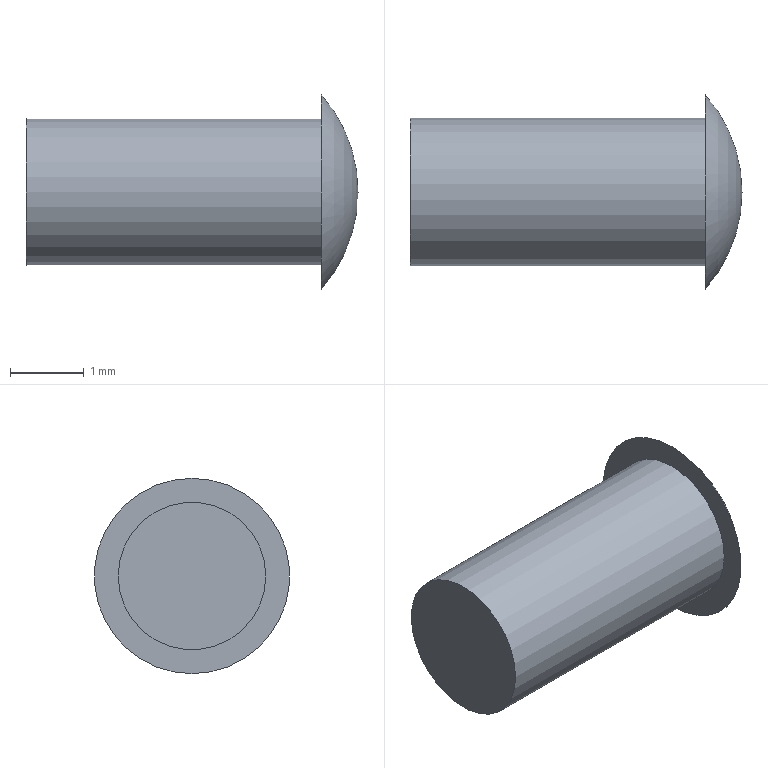Part | STEP file | 1-63部分2毫米Bolt | 1 solid | 4 faces | box 4.5 x 2.646 x 2.646 mm | volume 14.006 mm3 | plane 2 | cylinder 1 | sphere 1 | commonest cylinder face diameters 2 x1
STEP:
#1=CARTESIAN_POINT('',(0.,0.,0.));
#2=DIRECTION('',(0.,0.,1.));
#3=DIRECTION('',(1.,0.,0.));
#4=AXIS2_PLACEMENT_3D('',#1,#2,#3);
#5=CARTESIAN_POINT('',(-2.,1.,0.));
#6=VERTEX_POINT('',#5);
#7=CARTESIAN_POINT('',(-2.,0.,0.));
#8=DIRECTION('',(1.,0.,0.));
#9=DIRECTION('',(0.,1.,0.));
#10=AXIS2_PLACEMENT_3D('',#7,#8,#9);
#11=CIRCLE('',#10,1.);
#12=CARTESIAN_POINT('',(-2.,-0.2679,0.));
#13=DIRECTION('',(1.,0.,0.));
#14=DIRECTION('',(0.,1.,0.));
#15=AXIS2_PLACEMENT_3D('',#12,#13,#14);
#16=PLANE('',#15);
#17=CARTESIAN_POINT('',(0.2679,0.));
#18=DIRECTION('',(1.,0.));
#19=AXIS2_PLACEMENT_2D('',#17,#18);
#20=CIRCLE('',#19,1.);
#21=(GEOMETRIC_REPRESENTATION_CONTEXT(2)PARAMETRIC_REPRESENTATION_CONTEXT()REPRESENTATION_CONTEXT('',''));
#22=DEFINITIONAL_REPRESENTATION('',(#20),#21);
#23=PCURVE('',#16,#22);
#24=CARTESIAN_POINT('',(2.,0.,0.));
#25=DIRECTION('',(-1.,0.,0.));
#26=DIRECTION('',(0.,1.,0.));
#27=AXIS2_PLACEMENT_3D('',#24,#25,#26);
#28=CYLINDRICAL_SURFACE('',#27,1.);
#29=CARTESIAN_POINT('',(6.283,4.));
#30=DIRECTION('',(-1.,0.));
#31=VECTOR('',#30,1.);
#32=LINE('',#29,#31);
#33=(GEOMETRIC_REPRESENTATION_CONTEXT(2)PARAMETRIC_REPRESENTATION_CONTEXT()REPRESENTATION_CONTEXT('',''));
#34=DEFINITIONAL_REPRESENTATION('',(#32),#33);
#35=PCURVE('',#28,#34);
#36=SURFACE_CURVE('',#11,(#23,#35),.PCURVE_S1.);
#37=EDGE_CURVE('',#6,#6,#36,.T.);
#38=ORIENTED_EDGE('',*,*,#37,.T.);
#39=EDGE_LOOP('',(#38));
#40=FACE_BOUND('',#39,.F.);
#41=ADVANCED_FACE('',(#40),#16,.F.);
#42=CARTESIAN_POINT('',(2.,1.,0.));
#43=VERTEX_POINT('',#42);
#44=CARTESIAN_POINT('',(2.,1.,0.));
#45=DIRECTION('',(-1.,0.,0.));
#46=VECTOR('',#45,1.);
#47=LINE('',#44,#46);
#48=CARTESIAN_POINT('',(6.283,0.));
#49=DIRECTION('',(0.,1.));
#50=VECTOR('',#49,1.);
#51=LINE('',#48,#50);
#52=(GEOMETRIC_REPRESENTATION_CONTEXT(2)PARAMETRIC_REPRESENTATION_CONTEXT()REPRESENTATION_CONTEXT('',''));
#53=DEFINITIONAL_REPRESENTATION('',(#51),#52);
#54=PCURVE('',#28,#53);
#55=CARTESIAN_POINT('',(0.,0.));
#56=DIRECTION('',(0.,1.));
#57=VECTOR('',#56,1.);
#58=LINE('',#55,#57);
#59=(GEOMETRIC_REPRESENTATION_CONTEXT(2)PARAMETRIC_REPRESENTATION_CONTEXT()REPRESENTATION_CONTEXT('',''));
#60=DEFINITIONAL_REPRESENTATION('',(#58),#59);
#61=PCURVE('',#28,#60);
#62=SEAM_CURVE('',#47,(#54,#61),.PCURVE_S1.);
#63=EDGE_CURVE('',#43,#6,#62,.T.);
#64=ORIENTED_EDGE('',*,*,#63,.T.);
#65=ORIENTED_EDGE('',*,*,#37,.T.);
#66=ORIENTED_EDGE('',*,*,#63,.F.);
#67=CARTESIAN_POINT('',(2.,0.,0.));
#68=DIRECTION('',(1.,0.,0.));
#69=DIRECTION('',(0.,1.,0.));
#70=AXIS2_PLACEMENT_3D('',#67,#68,#69);
#71=CIRCLE('',#70,1.);
#72=CARTESIAN_POINT('',(6.283,0.));
#73=DIRECTION('',(-1.,0.));
#74=VECTOR('',#73,1.);
#75=LINE('',#72,#74);
#76=(GEOMETRIC_REPRESENTATION_CONTEXT(2)PARAMETRIC_REPRESENTATION_CONTEXT()REPRESENTATION_CONTEXT('',''));
#77=DEFINITIONAL_REPRESENTATION('',(#75),#76);
#78=PCURVE('',#28,#77);
#79=CARTESIAN_POINT('',(2.,0.,0.));
#80=DIRECTION('',(-1.,0.,0.));
#81=DIRECTION('',(0.,0.,1.));
#82=AXIS2_PLACEMENT_3D('',#79,#80,#81);
#83=PLANE('',#82);
#84=CARTESIAN_POINT('',(0.,1.));
#85=CARTESIAN_POINT('',(1.732,1.));
#86=CARTESIAN_POINT('',(0.866,-0.5));
#87=CARTESIAN_POINT('',(0.,-2.));
#88=CARTESIAN_POINT('',(-0.866,-0.5));
#89=CARTESIAN_POINT('',(-1.732,1.));
#90=CARTESIAN_POINT('',(0.,1.));
#91=(BOUNDED_CURVE()B_SPLINE_CURVE(2,(#84,#85,#86,#87,#88,#89,#90),.UNSPECIFIED.,.T.,.F.)B_SPLINE_CURVE_WITH_KNOTS((1,2,2,2,2,1),(-2.094,0.,2.094,4.189,6.283,8.378),.UNSPECIFIED.)CURVE()GEOMETRIC_REPRESENTATION_ITEM()RATIONAL_B_SPLINE_CURVE((1.,0.5,1.,0.5,1.,0.5,1.))REPRESENTATION_ITEM(''));
#92=(GEOMETRIC_REPRESENTATION_CONTEXT(2)PARAMETRIC_REPRESENTATION_CONTEXT()REPRESENTATION_CONTEXT('',''));
#93=DEFINITIONAL_REPRESENTATION('',(#91),#92);
#94=PCURVE('',#83,#93);
#95=SURFACE_CURVE('',#71,(#78,#94),.PCURVE_S1.);
#96=EDGE_CURVE('',#43,#43,#95,.T.);
#97=ORIENTED_EDGE('',*,*,#96,.F.);
#98=EDGE_LOOP('',(#64,#65,#66,#97));
#99=FACE_BOUND('',#98,.T.);
#100=ADVANCED_FACE('',(#99),#28,.T.);
#101=CARTESIAN_POINT('',(2.,0.,1.323));
#102=VERTEX_POINT('',#101);
#103=CARTESIAN_POINT('',(2.,0.,0.));
#104=DIRECTION('',(1.,0.,0.));
#105=DIRECTION('',(0.,0.,1.));
#106=AXIS2_PLACEMENT_3D('',#103,#104,#105);
#107=CIRCLE('',#106,1.323);
#108=CARTESIAN_POINT('',(1.323,0.));
#109=CARTESIAN_POINT('',(1.323,-2.291));
#110=CARTESIAN_POINT('',(-0.6614,-1.146));
#111=CARTESIAN_POINT('',(-2.646,0.));
#112=CARTESIAN_POINT('',(-0.6614,1.146));
#113=CARTESIAN_POINT('',(1.323,2.291));
#114=CARTESIAN_POINT('',(1.323,0.));
#115=(BOUNDED_CURVE()B_SPLINE_CURVE(2,(#108,#109,#110,#111,#112,#113,#114),.UNSPECIFIED.,.T.,.F.)B_SPLINE_CURVE_WITH_KNOTS((1,2,2,2,2,1),(-2.094,0.,2.094,4.189,6.283,8.378),.UNSPECIFIED.)CURVE()GEOMETRIC_REPRESENTATION_ITEM()RATIONAL_B_SPLINE_CURVE((1.,0.5,1.,0.5,1.,0.5,1.))REPRESENTATION_ITEM(''));
#116=(GEOMETRIC_REPRESENTATION_CONTEXT(2)PARAMETRIC_REPRESENTATION_CONTEXT()REPRESENTATION_CONTEXT('',''));
#117=DEFINITIONAL_REPRESENTATION('',(#115),#116);
#118=PCURVE('',#83,#117);
#119=CARTESIAN_POINT('',(0.5,0.,0.));
#120=DIRECTION('',(1.,0.,0.));
#121=DIRECTION('',(0.,0.,1.));
#122=AXIS2_PLACEMENT_3D('',#119,#120,#121);
#123=SPHERICAL_SURFACE('',#122,2.);
#124=CARTESIAN_POINT('',(0.,0.8481));
#125=CARTESIAN_POINT('',(0.0952,0.8481));
#126=CARTESIAN_POINT('',(0.2856,0.8481));
#127=CARTESIAN_POINT('',(0.5712,0.8481));
#128=CARTESIAN_POINT('',(0.8568,0.8481));
#129=CARTESIAN_POINT('',(1.142,0.8481));
#130=CARTESIAN_POINT('',(1.428,0.8481));
#131=CARTESIAN_POINT('',(1.714,0.8481));
#132=CARTESIAN_POINT('',(1.999,0.8481));
#133=CARTESIAN_POINT('',(2.285,0.8481));
#134=CARTESIAN_POINT('',(2.57,0.8481));
#135=CARTESIAN_POINT('',(2.856,0.8481));
#136=CARTESIAN_POINT('',(3.142,0.8481));
#137=CARTESIAN_POINT('',(3.427,0.8481));
#138=CARTESIAN_POINT('',(3.713,0.8481));
#139=CARTESIAN_POINT('',(3.998,0.8481));
#140=CARTESIAN_POINT('',(4.284,0.8481));
#141=CARTESIAN_POINT('',(4.57,0.8481));
#142=CARTESIAN_POINT('',(4.855,0.8481));
#143=CARTESIAN_POINT('',(5.141,0.8481));
#144=CARTESIAN_POINT('',(5.426,0.8481));
#145=CARTESIAN_POINT('',(5.712,0.8481));
#146=CARTESIAN_POINT('',(5.998,0.8481));
#147=CARTESIAN_POINT('',(6.188,0.8481));
#148=CARTESIAN_POINT('',(6.283,0.8481));
#149=B_SPLINE_CURVE_WITH_KNOTS('',3,(#124,#125,#126,#127,#128,#129,#130,#131,#132,#133,#134,#135,#136,#137,#138,#139,#140,#141,#142,#143,#144,#145,#146,#147,#148),.UNSPECIFIED.,.F.,.F.,(4,1,1,1,1,1,1,1,1,1,1,1,1,1,1,1,1,1,1,1,1,1,4),(0.,0.2856,0.5712,0.8568,1.142,1.428,1.714,1.999,2.285,2.57,2.856,3.142,3.427,3.713,3.998,4.284,4.57,4.855,5.141,5.426,5.712,5.998,6.283),.QUASI_UNIFORM_KNOTS.);
#150=(GEOMETRIC_REPRESENTATION_CONTEXT(2)PARAMETRIC_REPRESENTATION_CONTEXT()REPRESENTATION_CONTEXT('',''));
#151=DEFINITIONAL_REPRESENTATION('',(#149),#150);
#152=PCURVE('',#123,#151);
#153=SURFACE_CURVE('',#107,(#118,#152),.PCURVE_S1.);
#154=EDGE_CURVE('',#102,#102,#153,.T.);
#155=ORIENTED_EDGE('',*,*,#154,.F.);
#156=EDGE_LOOP('',(#155));
#157=FACE_BOUND('',#156,.T.);
#158=ORIENTED_EDGE('',*,*,#96,.T.);
#159=EDGE_LOOP('',(#158));
#160=FACE_BOUND('',#159,.T.);
#161=ADVANCED_FACE('',(#157,#160),#83,.T.);
#162=CARTESIAN_POINT('',(2.5,0.,0.));
#163=VERTEX_POINT('',#162);
#164=CARTESIAN_POINT('',(0.5,0.,0.));
#165=DIRECTION('',(0.,-1.,0.));
#166=DIRECTION('',(1.,0.,0.));
#167=AXIS2_PLACEMENT_3D('',#164,#165,#166);
#168=CIRCLE('',#167,2.);
#169=CARTESIAN_POINT('',(0.,1.571));
#170=CARTESIAN_POINT('',(0.,1.56));
#171=CARTESIAN_POINT('',(0.,1.538));
#172=CARTESIAN_POINT('',(0.,1.505));
#173=CARTESIAN_POINT('',(0.,1.472));
#174=CARTESIAN_POINT('',(0.,1.439));
#175=CARTESIAN_POINT('',(0.,1.407));
#176=CARTESIAN_POINT('',(0.,1.374));
#177=CARTESIAN_POINT('',(0.,1.341));
#178=CARTESIAN_POINT('',(0.,1.308));
#179=CARTESIAN_POINT('',(0.,1.275));
#180=CARTESIAN_POINT('',(0.,1.242));
#181=CARTESIAN_POINT('',(0.,1.209));
#182=CARTESIAN_POINT('',(0.,1.177));
#183=CARTESIAN_POINT('',(0.,1.144));
#184=CARTESIAN_POINT('',(0.,1.111));
#185=CARTESIAN_POINT('',(0.,1.078));
#186=CARTESIAN_POINT('',(0.,1.045));
#187=CARTESIAN_POINT('',(0.,1.012));
#188=CARTESIAN_POINT('',(0.,0.9795));
#189=CARTESIAN_POINT('',(0.,0.9466));
#190=CARTESIAN_POINT('',(0.,0.9138));
#191=CARTESIAN_POINT('',(0.,0.8809));
#192=CARTESIAN_POINT('',(0.,0.859));
#193=CARTESIAN_POINT('',(0.,0.8481));
#194=B_SPLINE_CURVE_WITH_KNOTS('',3,(#169,#170,#171,#172,#173,#174,#175,#176,#177,#178,#179,#180,#181,#182,#183,#184,#185,#186,#187,#188,#189,#190,#191,#192,#193),.UNSPECIFIED.,.F.,.F.,(4,1,1,1,1,1,1,1,1,1,1,1,1,1,1,1,1,1,1,1,1,1,4),(0.,0.03285,0.0657,0.09855,0.1314,0.1643,0.1971,0.23,0.2628,0.2957,0.3285,0.3614,0.3942,0.4271,0.4599,0.4928,0.5256,0.5585,0.5913,0.6242,0.657,0.6899,0.7227),.QUASI_UNIFORM_KNOTS.);
#195=(GEOMETRIC_REPRESENTATION_CONTEXT(2)PARAMETRIC_REPRESENTATION_CONTEXT()REPRESENTATION_CONTEXT('',''));
#196=DEFINITIONAL_REPRESENTATION('',(#194),#195);
#197=PCURVE('',#123,#196);
#198=CARTESIAN_POINT('',(6.283,1.571));
#199=CARTESIAN_POINT('',(6.283,1.56));
#200=CARTESIAN_POINT('',(6.283,1.538));
#201=CARTESIAN_POINT('',(6.283,1.505));
#202=CARTESIAN_POINT('',(6.283,1.472));
#203=CARTESIAN_POINT('',(6.283,1.439));
#204=CARTESIAN_POINT('',(6.283,1.407));
#205=CARTESIAN_POINT('',(6.283,1.374));
#206=CARTESIAN_POINT('',(6.283,1.341));
#207=CARTESIAN_POINT('',(6.283,1.308));
#208=CARTESIAN_POINT('',(6.283,1.275));
#209=CARTESIAN_POINT('',(6.283,1.242));
#210=CARTESIAN_POINT('',(6.283,1.209));
#211=CARTESIAN_POINT('',(6.283,1.177));
#212=CARTESIAN_POINT('',(6.283,1.144));
#213=CARTESIAN_POINT('',(6.283,1.111));
#214=CARTESIAN_POINT('',(6.283,1.078));
#215=CARTESIAN_POINT('',(6.283,1.045));
#216=CARTESIAN_POINT('',(6.283,1.012));
#217=CARTESIAN_POINT('',(6.283,0.9795));
#218=CARTESIAN_POINT('',(6.283,0.9466));
#219=CARTESIAN_POINT('',(6.283,0.9138));
#220=CARTESIAN_POINT('',(6.283,0.8809));
#221=CARTESIAN_POINT('',(6.283,0.859));
#222=CARTESIAN_POINT('',(6.283,0.8481));
#223=B_SPLINE_CURVE_WITH_KNOTS('',3,(#198,#199,#200,#201,#202,#203,#204,#205,#206,#207,#208,#209,#210,#211,#212,#213,#214,#215,#216,#217,#218,#219,#220,#221,#222),.UNSPECIFIED.,.F.,.F.,(4,1,1,1,1,1,1,1,1,1,1,1,1,1,1,1,1,1,1,1,1,1,4),(0.,0.03285,0.0657,0.09855,0.1314,0.1643,0.1971,0.23,0.2628,0.2957,0.3285,0.3614,0.3942,0.4271,0.4599,0.4928,0.5256,0.5585,0.5913,0.6242,0.657,0.6899,0.7227),.QUASI_UNIFORM_KNOTS.);
#224=(GEOMETRIC_REPRESENTATION_CONTEXT(2)PARAMETRIC_REPRESENTATION_CONTEXT()REPRESENTATION_CONTEXT('',''));
#225=DEFINITIONAL_REPRESENTATION('',(#223),#224);
#226=PCURVE('',#123,#225);
#227=SEAM_CURVE('',#168,(#197,#226),.PCURVE_S1.);
#228=EDGE_CURVE('',#163,#102,#227,.T.);
#229=ORIENTED_EDGE('',*,*,#228,.T.);
#230=ORIENTED_EDGE('',*,*,#154,.T.);
#231=ORIENTED_EDGE('',*,*,#228,.F.);
#232=EDGE_LOOP('',(#229,#230,#231));
#233=FACE_BOUND('',#232,.T.);
#234=ADVANCED_FACE('',(#233),#123,.T.);
#235=CLOSED_SHELL('',(#41,#100,#161,#234));
#236=MANIFOLD_SOLID_BREP('',#235);
#237=(LENGTH_UNIT()NAMED_UNIT(*)SI_UNIT(.MILLI.,.METRE.));
#238=UNCERTAINTY_MEASURE_WITH_UNIT(LENGTH_MEASURE(0.0000001),#237,'','');
#239=(NAMED_UNIT(*)PLANE_ANGLE_UNIT()SI_UNIT($,.RADIAN.));
#240=(NAMED_UNIT(*)SI_UNIT($,.STERADIAN.)SOLID_ANGLE_UNIT());
#241=(GEOMETRIC_REPRESENTATION_CONTEXT(3)GLOBAL_UNCERTAINTY_ASSIGNED_CONTEXT((#238))GLOBAL_UNIT_ASSIGNED_CONTEXT((#237,#239,#240))REPRESENTATION_CONTEXT('',''));
#242=ADVANCED_BREP_SHAPE_REPRESENTATION('',(#4,#236),#241);